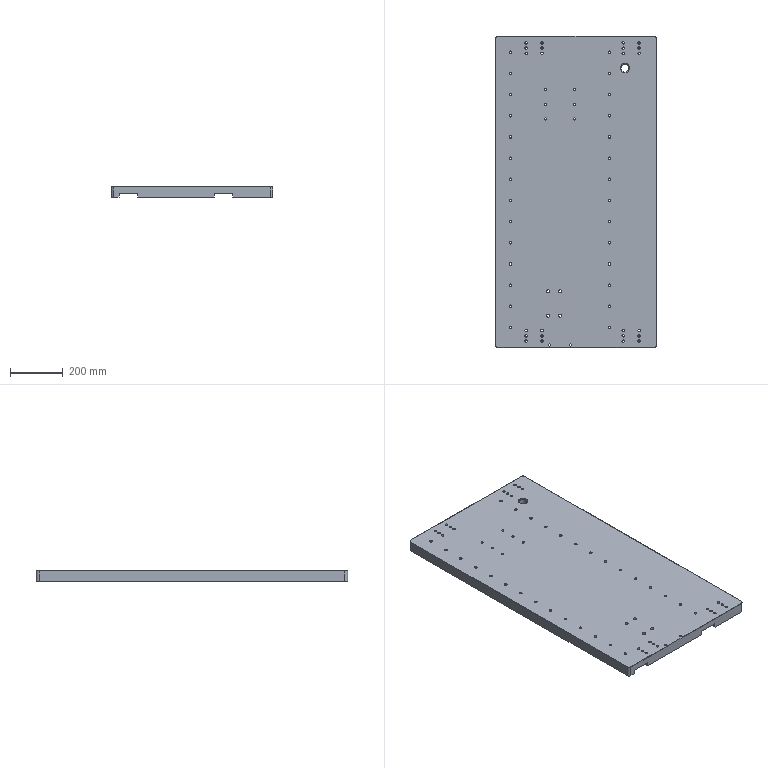Part | SolidWorks | features HoleWzd 4, ICE 2, BaseBody 1, MoveFace 1 | 1 solid | 398 faces | box 610 x 1176 x 40 mm | volume 25279408 mm3 | cylinder 190 | cone 140 | plane 68 | commonest cylinder face diameters 8.5 x72 9 x48 15 x48 12 x12 5.2 x4 20 x4